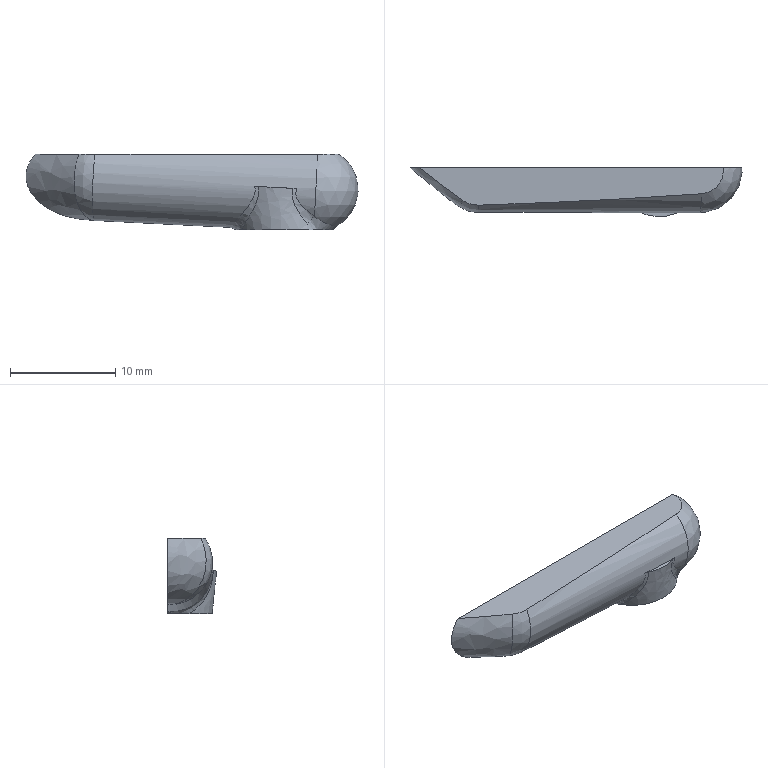Part | STEP file | solid 218 | 1 solid | 15 faces | box 31.5 x 4.648 x 7.129 mm | volume 682.585 mm3 | spline 9 | plane 4 | sphere 1 | cylinder 1 | commonest cylinder face diameters 8 x1